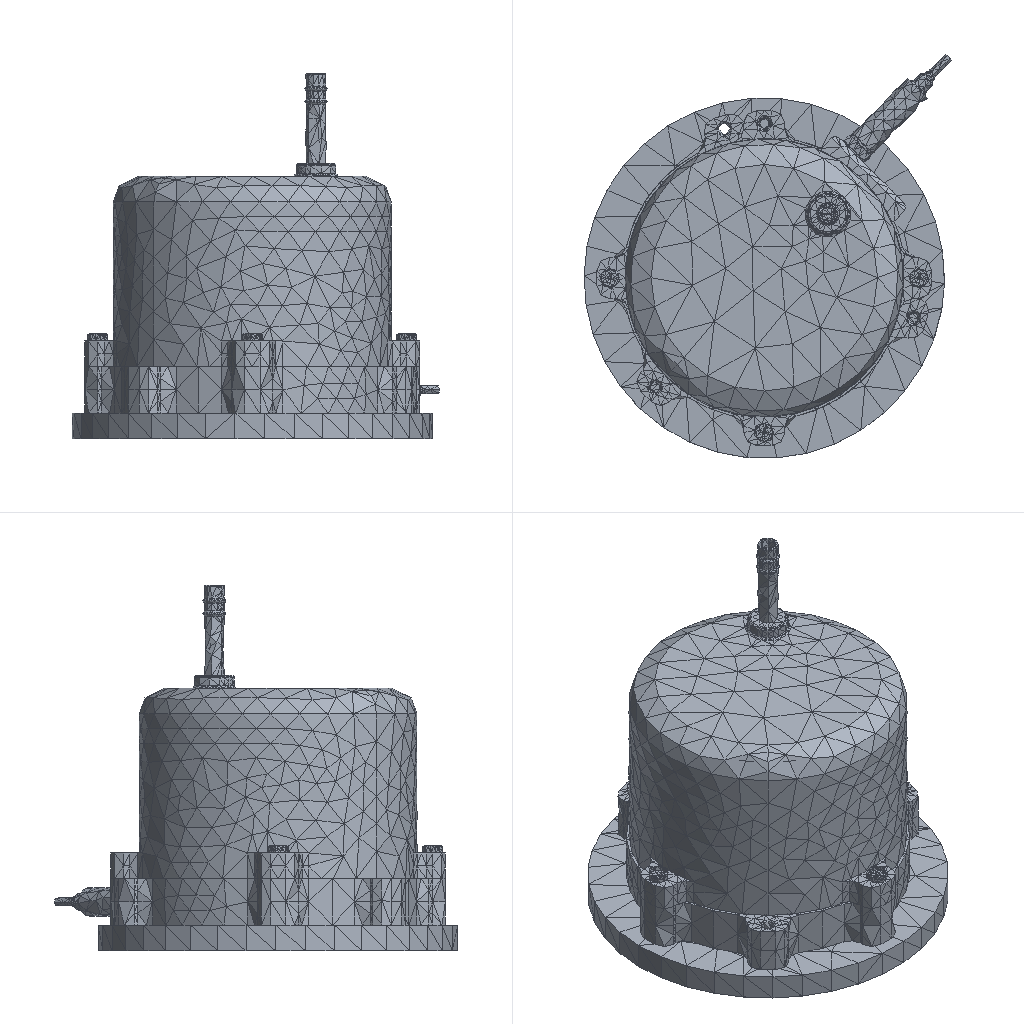Simulation study | ansys workbench
Ansys APDL input file, long lists of numbers shortened:
/batch
/config,noeldb,1     ! force off writing results to database
*get,_wallstrt,active,,time,wall
! ANSYS input file written by Workbench version 2022 R1
/com,*********** Resuming The ANSYS db File from Modal Solution ***********
resume,file,db
*DIM,_wb_ProjectScratch_dir_Harmonic,string,248
_wb_ProjectScratch_dir_Harmonic(1)= 'F:\____________________\__________________\_______________\_______\_
*DIM,_wb_SolverFiles_dir_Harmonic,string,248
_wb_SolverFiles_dir_Harmonic(1)= 'F:\____________________\__________________\________________________\___\_____\____\_
*DIM,_wb_userfiles_dir_Harmonic,string,248
_wb_userfiles_dir_Harmonic(1)= 'F:\____________________\__________________\________________________\__________\_
/title,_________--____ (C5)
! ****** Begin Custom Load Command Snippet ******
/COM, ACT Extensions:
/COM,     LSDYNA, 2021.1
/COM,
! ****** End   Custom Load Command Snippet ******
/nopr
/prep7
/com,*********** Defining Loadings ***********
/com,*********** Define Force Using Surface Effect Elements ***********
local,12,0,0.,0.,0.,0.,0.,0.
csys,0
et,137,154
eblock,10,,,84
(15i9)
   164210      137      137      137       12    38938    38946    38945    38945    45720    45748    38945    45719
! (83 more lines like these left out)
-1
esel,s,type,,137
keyop,137,2,1                ! Apply load in local coordinate system
keyop,137,7,1                ! Use original area so load is constant in large deformation
esel,all
*DIM,_loadvari358x,TABLE,1,1,1,TIME
! Time values
*TAXIS,_loadvari358x(1),1,1.
! Load values
_loadvari358x(1,1,1) = 0.
*DIM,_loadvari358xi,TABLE,1,1,1,TIME
! Time values
*TAXIS,_loadvari358xi(1),1,1.
! Load values
_loadvari358xi(1,1,1) = 0.
*DIM,_loadvari358y,TABLE,1,1,1,TIME
! Time values
*TAXIS,_loadvari358y(1),1,1.
! Load values
_loadvari358y(1,1,1) = 0.
*DIM,_loadvari358yi,TABLE,1,1,1,TIME
! Time values
*TAXIS,_loadvari358yi(1),1,1.
! Load values
_loadvari358yi(1,1,1) = 0.
*DIM,_loadvari358z,TABLE,1,1,1,TIME
! Time values
*TAXIS,_loadvari358z(1),1,1.
! Load values
_loadvari358z(1,1,1) = -1.71620860288242e-003
*DIM,_loadvari358zi,TABLE,1,1,1,TIME
! Time values
*TAXIS,_loadvari358zi(1),1,1.
! Load values
_loadvari358zi(1,1,1) = 0.
fini
/com,*********** Performing Modal Re-start ***********
/gopr
/solu
antype,modal,restart    ! restarting the modal analysis
modcontrol,on
thexpand,off     ! ignore thermal strains
mxpand,,,,yes,,yes     ! expand requested results and write them to file.mode
outres,erase
outres,all,none
outres,nsol,all
outres,eangl,all
outres,etmp,all
outres,veng,all
outres,strs,all
outres,epel,all
outres,rsol,all
outres,cont,all
fdele,all,all
sfdele,all,all
sfedele,all,all,all
acel,0,0,0                 ! zero out the acceleration
/com,*********** Setting and Solving Each Load Step ***********
esel,s,type,,137
nsle
sfe,all,3,pres,1,1
nsel,all
esel,all
solve
/com,**********************
/com *************** Write FE CONNECTORS *********
CEWRITE,file,ce,,INTE
fini
/com,*********** Performing MSUP Harmonic Solve ***********
/solu
antype,harm
hropt,msup
thexpand,off     ! ignore thermal strains
hrout,off,on
kbc,1
harfrq,380.,480.
nsub,4
fdele,all,all
sfdele,all,all
sfedele,all,all,all
acel,0,0,0                 ! zero out the acceleration
lvscale,0,1
/com,*********** Scaling Each Load Step for MSUP Solve ***********
lvscale,%_loadvari358z%,1
! *********** WB SOLVE COMMAND ***********
! check interactive state
*get,ANSINTER_,active,,int
*if,ANSINTER_,ne,0,then
/eof
*endif
solve
fini
*get,_wallasol,active,,time,wall
/nopr
*get,_numnode,node,0,count
*get,_numelem,elem,0,count
*get, _MAXELEMNUM, elem, 0, NUM, MAX
*get, _MAXNODENUM, node, 0, NUM, MAX,,,INTERNAL
*get, _MAXELEMTYPE, etyp, 0, NUM, MAX
*get, _MAXREALCONST, real, 0, NUM, MAX
/gopr
! ------- MSUP EXPANSION PASS -------
/solu
expass,on
hrexp,all
outres,erase
outres,all,none
outres,nsol,all
outres,eangl,all
outres,etmp,all
outres,veng,all
outres,strs,all
outres,epel,all
outres,rsol,all
outres,cont,all
numexp,all,,,yes        ! expand results at all freq. and calculate requested result items
! *********** WB SOLVE COMMAND ***********
! check interactive state
*get,ANSINTER_,active,,int
*if,ANSINTER_,ne,0,then
/eof
*endif
solve
fini
/post1
xmlo,ENCODING,ISO-8859-1
xmlo,parm
/xml,parm,xml
fini
/gopr
*get,_walldone,active,,time,wall
_preptime=(_wallbsol-_wallstrt)*3600
_solvtime=(_wallasol-_wallbsol)*3600
_posttime=(_walldone-_wallasol)*3600
_totaltim=(_walldone-_wallstrt)*3600
*get,_dlbratio,active,0,solu,dlbr
*get,_combtime,active,0,solu,comb
*get,_ssmode,active,0,solu,ssmm
*get,_ndofs,active,0,solu,ndof
/fclean				!clean distributed files
/com,--- Total number of nodes = %_numnode%
/com,--- Total number of elements = %_numelem%
/com,--- Element load balance ratio = %_dlbratio%
/com,--- Time to combine distributed files = %_combtime%
/com,--- Sparse memory mode = %_ssmode%
/com,--- Number of DOF = %_ndofs%
/wb,file,end               ! done with WB generated input